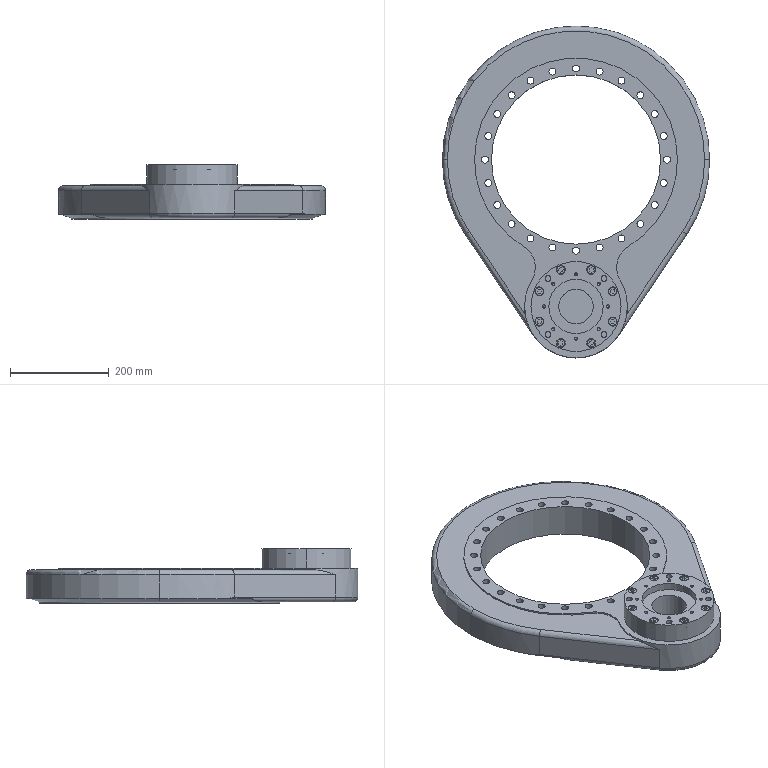Part | SolidWorks | features ICE 12, CirPattern 2, Chamfer 1, Extrusion 1, Fillet 1, HoleWzd 1, RevCut 1 | 1 solid | 316 faces | box 540 x 671 x 111 mm | volume 11365410 mm3 | cylinder 181 | plane 111 | cone 20 | torus 4 | commonest cylinder face diameters 10.6 x48 14 x48 6.6 x16 16 x16 18 x16 12 x8